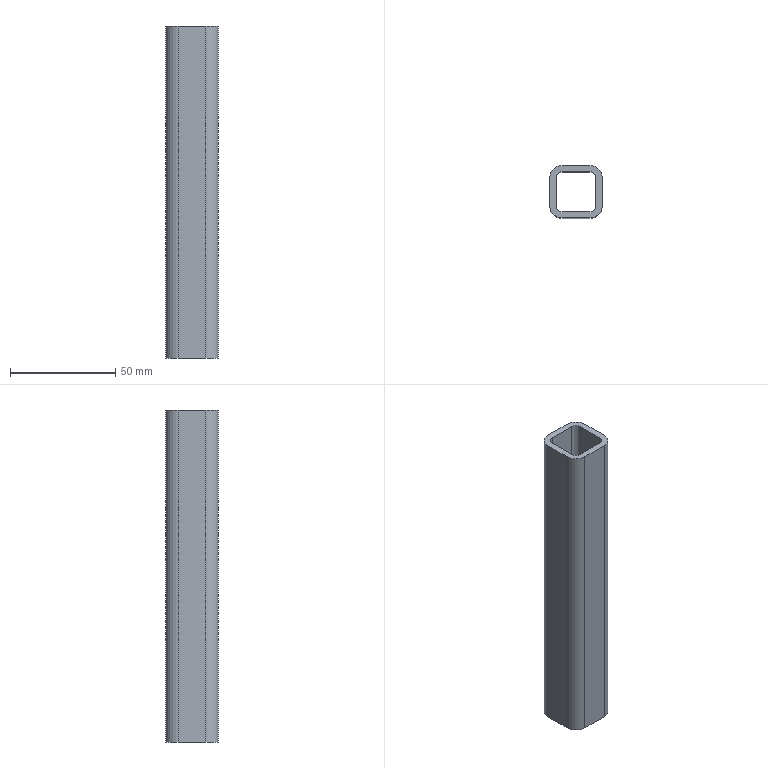Part | STEP file | ISO 10799-2 25x25x3 1784906820767 | 1 solid | 18 faces | box 25 x 25 x 158 mm | volume 38050 mm3 | plane 10 | cylinder 8 | commonest cylinder face diameters 6 x4 12 x4
STEP:
#1=CARTESIAN_POINT('',(-6.5,-9.5,183.));
#2=VERTEX_POINT('',#1);
#3=CARTESIAN_POINT('',(6.5,-9.5,183.));
#4=VERTEX_POINT('',#3);
#5=CARTESIAN_POINT('',(3.25,-9.5,183.));
#6=DIRECTION('',(1.,0.,0.));
#7=VECTOR('',#6,10.);
#8=LINE('',#5,#7);
#9=EDGE_CURVE('',#2,#4,#8,.T.);
#10=ORIENTED_EDGE('',*,*,#9,.T.);
#11=CARTESIAN_POINT('',(6.5,-9.5,25.));
#12=VERTEX_POINT('',#11);
#13=CARTESIAN_POINT('',(6.5,-9.5,0.));
#14=DIRECTION('',(0.,0.,1.));
#15=VECTOR('',#14,10.);
#16=LINE('',#13,#15);
#17=EDGE_CURVE('',#12,#4,#16,.T.);
#18=ORIENTED_EDGE('',*,*,#17,.F.);
#19=CARTESIAN_POINT('',(-6.5,-9.5,25.));
#20=VERTEX_POINT('',#19);
#21=CARTESIAN_POINT('',(3.25,-9.5,25.));
#22=DIRECTION('',(1.,0.,0.));
#23=VECTOR('',#22,10.);
#24=LINE('',#21,#23);
#25=EDGE_CURVE('',#20,#12,#24,.T.);
#26=ORIENTED_EDGE('',*,*,#25,.F.);
#27=CARTESIAN_POINT('',(-6.5,-9.5,0.));
#28=DIRECTION('',(0.,0.,1.));
#29=VECTOR('',#28,10.);
#30=LINE('',#27,#29);
#31=EDGE_CURVE('',#20,#2,#30,.T.);
#32=ORIENTED_EDGE('',*,*,#31,.T.);
#33=EDGE_LOOP('',(#10,#18,#26,#32));
#34=FACE_OUTER_BOUND('',#33,.T.);
#35=CARTESIAN_POINT('',(6.5,-9.5,0.));
#36=DIRECTION('',(0.,-1.,0.));
#37=DIRECTION('',(0.,0.,-1.));
#38=AXIS2_PLACEMENT_3D('',#35,#36,#37);
#39=PLANE('',#38);
#40=ADVANCED_FACE('',(#34),#39,.F.);
#41=CARTESIAN_POINT('',(9.5,-6.5,183.));
#42=VERTEX_POINT('',#41);
#43=CARTESIAN_POINT('',(6.5,-6.5,183.));
#44=DIRECTION('',(0.,0.,1.));
#45=DIRECTION('',(0.,1.,0.));
#46=AXIS2_PLACEMENT_3D('',#43,#44,#45);
#47=CIRCLE('',#46,3.);
#48=EDGE_CURVE('',#4,#42,#47,.T.);
#49=ORIENTED_EDGE('',*,*,#48,.T.);
#50=CARTESIAN_POINT('',(9.5,-6.5,25.));
#51=VERTEX_POINT('',#50);
#52=CARTESIAN_POINT('',(9.5,-6.5,0.));
#53=DIRECTION('',(0.,0.,1.));
#54=VECTOR('',#53,10.);
#55=LINE('',#52,#54);
#56=EDGE_CURVE('',#51,#42,#55,.T.);
#57=ORIENTED_EDGE('',*,*,#56,.F.);
#58=CARTESIAN_POINT('',(6.5,-6.5,25.));
#59=DIRECTION('',(0.,0.,1.));
#60=DIRECTION('',(0.,1.,0.));
#61=AXIS2_PLACEMENT_3D('',#58,#59,#60);
#62=CIRCLE('',#61,3.);
#63=EDGE_CURVE('',#12,#51,#62,.T.);
#64=ORIENTED_EDGE('',*,*,#63,.F.);
#65=ORIENTED_EDGE('',*,*,#17,.T.);
#66=EDGE_LOOP('',(#49,#57,#64,#65));
#67=FACE_OUTER_BOUND('',#66,.T.);
#68=CARTESIAN_POINT('',(6.5,-6.5,0.));
#69=DIRECTION('',(0.,0.,1.));
#70=DIRECTION('',(0.,1.,0.));
#71=AXIS2_PLACEMENT_3D('',#68,#69,#70);
#72=CYLINDRICAL_SURFACE('',#71,3.);
#73=ADVANCED_FACE('',(#67),#72,.F.);
#74=CARTESIAN_POINT('',(9.5,6.5,183.));
#75=VERTEX_POINT('',#74);
#76=CARTESIAN_POINT('',(9.5,3.25,183.));
#77=DIRECTION('',(0.,1.,0.));
#78=VECTOR('',#77,10.);
#79=LINE('',#76,#78);
#80=EDGE_CURVE('',#42,#75,#79,.T.);
#81=ORIENTED_EDGE('',*,*,#80,.T.);
#82=CARTESIAN_POINT('',(9.5,6.5,25.));
#83=VERTEX_POINT('',#82);
#84=CARTESIAN_POINT('',(9.5,6.5,0.));
#85=DIRECTION('',(0.,0.,1.));
#86=VECTOR('',#85,10.);
#87=LINE('',#84,#86);
#88=EDGE_CURVE('',#83,#75,#87,.T.);
#89=ORIENTED_EDGE('',*,*,#88,.F.);
#90=CARTESIAN_POINT('',(9.5,3.25,25.));
#91=DIRECTION('',(0.,1.,0.));
#92=VECTOR('',#91,10.);
#93=LINE('',#90,#92);
#94=EDGE_CURVE('',#51,#83,#93,.T.);
#95=ORIENTED_EDGE('',*,*,#94,.F.);
#96=ORIENTED_EDGE('',*,*,#56,.T.);
#97=EDGE_LOOP('',(#81,#89,#95,#96));
#98=FACE_OUTER_BOUND('',#97,.T.);
#99=CARTESIAN_POINT('',(9.5,6.5,0.));
#100=DIRECTION('',(1.,0.,0.));
#101=DIRECTION('',(0.,0.,-1.));
#102=AXIS2_PLACEMENT_3D('',#99,#100,#101);
#103=PLANE('',#102);
#104=ADVANCED_FACE('',(#98),#103,.F.);
#105=CARTESIAN_POINT('',(6.5,9.5,183.));
#106=VERTEX_POINT('',#105);
#107=CARTESIAN_POINT('',(6.5,6.5,183.));
#108=DIRECTION('',(0.,0.,1.));
#109=DIRECTION('',(-1.,0.,0.));
#110=AXIS2_PLACEMENT_3D('',#107,#108,#109);
#111=CIRCLE('',#110,3.);
#112=EDGE_CURVE('',#75,#106,#111,.T.);
#113=ORIENTED_EDGE('',*,*,#112,.T.);
#114=CARTESIAN_POINT('',(6.5,9.5,25.));
#115=VERTEX_POINT('',#114);
#116=CARTESIAN_POINT('',(6.5,9.5,0.));
#117=DIRECTION('',(0.,0.,1.));
#118=VECTOR('',#117,10.);
#119=LINE('',#116,#118);
#120=EDGE_CURVE('',#115,#106,#119,.T.);
#121=ORIENTED_EDGE('',*,*,#120,.F.);
#122=CARTESIAN_POINT('',(6.5,6.5,25.));
#123=DIRECTION('',(0.,0.,1.));
#124=DIRECTION('',(-1.,0.,0.));
#125=AXIS2_PLACEMENT_3D('',#122,#123,#124);
#126=CIRCLE('',#125,3.);
#127=EDGE_CURVE('',#83,#115,#126,.T.);
#128=ORIENTED_EDGE('',*,*,#127,.F.);
#129=ORIENTED_EDGE('',*,*,#88,.T.);
#130=EDGE_LOOP('',(#113,#121,#128,#129));
#131=FACE_OUTER_BOUND('',#130,.T.);
#132=CARTESIAN_POINT('',(6.5,6.5,0.));
#133=DIRECTION('',(0.,0.,1.));
#134=DIRECTION('',(-1.,0.,0.));
#135=AXIS2_PLACEMENT_3D('',#132,#133,#134);
#136=CYLINDRICAL_SURFACE('',#135,3.);
#137=ADVANCED_FACE('',(#131),#136,.F.);
#138=CARTESIAN_POINT('',(12.5,6.5,183.));
#139=VERTEX_POINT('',#138);
#140=CARTESIAN_POINT('',(12.5,-6.5,183.));
#141=VERTEX_POINT('',#140);
#142=CARTESIAN_POINT('',(12.5,3.25,183.));
#143=DIRECTION('',(0.,-1.,0.));
#144=VECTOR('',#143,10.);
#145=LINE('',#142,#144);
#146=EDGE_CURVE('',#139,#141,#145,.T.);
#147=ORIENTED_EDGE('',*,*,#146,.T.);
#148=CARTESIAN_POINT('',(12.5,-6.5,25.));
#149=VERTEX_POINT('',#148);
#150=CARTESIAN_POINT('',(12.5,-6.5,0.));
#151=DIRECTION('',(0.,0.,1.));
#152=VECTOR('',#151,10.);
#153=LINE('',#150,#152);
#154=EDGE_CURVE('',#149,#141,#153,.T.);
#155=ORIENTED_EDGE('',*,*,#154,.F.);
#156=CARTESIAN_POINT('',(12.5,6.5,25.));
#157=VERTEX_POINT('',#156);
#158=CARTESIAN_POINT('',(12.5,3.25,25.));
#159=DIRECTION('',(0.,-1.,0.));
#160=VECTOR('',#159,10.);
#161=LINE('',#158,#160);
#162=EDGE_CURVE('',#157,#149,#161,.T.);
#163=ORIENTED_EDGE('',*,*,#162,.F.);
#164=CARTESIAN_POINT('',(12.5,6.5,0.));
#165=DIRECTION('',(0.,0.,1.));
#166=VECTOR('',#165,10.);
#167=LINE('',#164,#166);
#168=EDGE_CURVE('',#157,#139,#167,.T.);
#169=ORIENTED_EDGE('',*,*,#168,.T.);
#170=EDGE_LOOP('',(#147,#155,#163,#169));
#171=FACE_OUTER_BOUND('',#170,.T.);
#172=CARTESIAN_POINT('',(12.5,6.5,0.));
#173=DIRECTION('',(1.,0.,0.));
#174=DIRECTION('',(0.,0.,-1.));
#175=AXIS2_PLACEMENT_3D('',#172,#173,#174);
#176=PLANE('',#175);
#177=ADVANCED_FACE('',(#171),#176,.T.);
#178=CARTESIAN_POINT('',(6.5,-12.5,183.));
#179=VERTEX_POINT('',#178);
#180=CARTESIAN_POINT('',(6.5,-6.5,183.));
#181=DIRECTION('',(0.,0.,-1.));
#182=DIRECTION('',(0.,1.,0.));
#183=AXIS2_PLACEMENT_3D('',#180,#181,#182);
#184=CIRCLE('',#183,6.);
#185=EDGE_CURVE('',#141,#179,#184,.T.);
#186=ORIENTED_EDGE('',*,*,#185,.T.);
#187=CARTESIAN_POINT('',(6.5,-12.5,25.));
#188=VERTEX_POINT('',#187);
#189=CARTESIAN_POINT('',(6.5,-12.5,0.));
#190=DIRECTION('',(0.,0.,1.));
#191=VECTOR('',#190,10.);
#192=LINE('',#189,#191);
#193=EDGE_CURVE('',#188,#179,#192,.T.);
#194=ORIENTED_EDGE('',*,*,#193,.F.);
#195=CARTESIAN_POINT('',(6.5,-6.5,25.));
#196=DIRECTION('',(0.,0.,-1.));
#197=DIRECTION('',(0.,1.,0.));
#198=AXIS2_PLACEMENT_3D('',#195,#196,#197);
#199=CIRCLE('',#198,6.);
#200=EDGE_CURVE('',#149,#188,#199,.T.);
#201=ORIENTED_EDGE('',*,*,#200,.F.);
#202=ORIENTED_EDGE('',*,*,#154,.T.);
#203=EDGE_LOOP('',(#186,#194,#201,#202));
#204=FACE_OUTER_BOUND('',#203,.T.);
#205=CARTESIAN_POINT('',(6.5,-6.5,0.));
#206=DIRECTION('',(0.,0.,1.));
#207=DIRECTION('',(0.,1.,0.));
#208=AXIS2_PLACEMENT_3D('',#205,#206,#207);
#209=CYLINDRICAL_SURFACE('',#208,6.);
#210=ADVANCED_FACE('',(#204),#209,.T.);
#211=CARTESIAN_POINT('',(-6.5,-12.5,183.));
#212=VERTEX_POINT('',#211);
#213=CARTESIAN_POINT('',(3.25,-12.5,183.));
#214=DIRECTION('',(-1.,0.,0.));
#215=VECTOR('',#214,10.);
#216=LINE('',#213,#215);
#217=EDGE_CURVE('',#179,#212,#216,.T.);
#218=ORIENTED_EDGE('',*,*,#217,.T.);
#219=CARTESIAN_POINT('',(-6.5,-12.5,25.));
#220=VERTEX_POINT('',#219);
#221=CARTESIAN_POINT('',(-6.5,-12.5,0.));
#222=DIRECTION('',(0.,0.,1.));
#223=VECTOR('',#222,10.);
#224=LINE('',#221,#223);
#225=EDGE_CURVE('',#220,#212,#224,.T.);
#226=ORIENTED_EDGE('',*,*,#225,.F.);
#227=CARTESIAN_POINT('',(3.25,-12.5,25.));
#228=DIRECTION('',(-1.,0.,0.));
#229=VECTOR('',#228,10.);
#230=LINE('',#227,#229);
#231=EDGE_CURVE('',#188,#220,#230,.T.);
#232=ORIENTED_EDGE('',*,*,#231,.F.);
#233=ORIENTED_EDGE('',*,*,#193,.T.);
#234=EDGE_LOOP('',(#218,#226,#232,#233));
#235=FACE_OUTER_BOUND('',#234,.T.);
#236=CARTESIAN_POINT('',(6.5,-12.5,0.));
#237=DIRECTION('',(0.,-1.,0.));
#238=DIRECTION('',(0.,0.,-1.));
#239=AXIS2_PLACEMENT_3D('',#236,#237,#238);
#240=PLANE('',#239);
#241=ADVANCED_FACE('',(#235),#240,.T.);
#242=CARTESIAN_POINT('',(-12.5,-6.5,183.));
#243=VERTEX_POINT('',#242);
#244=CARTESIAN_POINT('',(-6.5,-6.5,183.));
#245=DIRECTION('',(0.,0.,-1.));
#246=DIRECTION('',(1.,0.,0.));
#247=AXIS2_PLACEMENT_3D('',#244,#245,#246);
#248=CIRCLE('',#247,6.);
#249=EDGE_CURVE('',#212,#243,#248,.T.);
#250=ORIENTED_EDGE('',*,*,#249,.T.);
#251=CARTESIAN_POINT('',(-12.5,-6.5,25.));
#252=VERTEX_POINT('',#251);
#253=CARTESIAN_POINT('',(-12.5,-6.5,0.));
#254=DIRECTION('',(0.,0.,1.));
#255=VECTOR('',#254,10.);
#256=LINE('',#253,#255);
#257=EDGE_CURVE('',#252,#243,#256,.T.);
#258=ORIENTED_EDGE('',*,*,#257,.F.);
#259=CARTESIAN_POINT('',(-6.5,-6.5,25.));
#260=DIRECTION('',(0.,0.,-1.));
#261=DIRECTION('',(1.,0.,0.));
#262=AXIS2_PLACEMENT_3D('',#259,#260,#261);
#263=CIRCLE('',#262,6.);
#264=EDGE_CURVE('',#220,#252,#263,.T.);
#265=ORIENTED_EDGE('',*,*,#264,.F.);
#266=ORIENTED_EDGE('',*,*,#225,.T.);
#267=EDGE_LOOP('',(#250,#258,#265,#266));
#268=FACE_OUTER_BOUND('',#267,.T.);
#269=CARTESIAN_POINT('',(-6.5,-6.5,0.));
#270=DIRECTION('',(0.,0.,1.));
#271=DIRECTION('',(1.,0.,0.));
#272=AXIS2_PLACEMENT_3D('',#269,#270,#271);
#273=CYLINDRICAL_SURFACE('',#272,6.);
#274=ADVANCED_FACE('',(#268),#273,.T.);
#275=CARTESIAN_POINT('',(-6.5,9.5,183.));
#276=VERTEX_POINT('',#275);
#277=CARTESIAN_POINT('',(-3.25,9.5,183.));
#278=DIRECTION('',(-1.,0.,0.));
#279=VECTOR('',#278,10.);
#280=LINE('',#277,#279);
#281=EDGE_CURVE('',#106,#276,#280,.T.);
#282=ORIENTED_EDGE('',*,*,#281,.T.);
#283=CARTESIAN_POINT('',(-6.5,9.5,25.));
#284=VERTEX_POINT('',#283);
#285=CARTESIAN_POINT('',(-6.5,9.5,0.));
#286=DIRECTION('',(0.,0.,1.));
#287=VECTOR('',#286,10.);
#288=LINE('',#285,#287);
#289=EDGE_CURVE('',#284,#276,#288,.T.);
#290=ORIENTED_EDGE('',*,*,#289,.F.);
#291=CARTESIAN_POINT('',(-3.25,9.5,25.));
#292=DIRECTION('',(-1.,0.,0.));
#293=VECTOR('',#292,10.);
#294=LINE('',#291,#293);
#295=EDGE_CURVE('',#115,#284,#294,.T.);
#296=ORIENTED_EDGE('',*,*,#295,.F.);
#297=ORIENTED_EDGE('',*,*,#120,.T.);
#298=EDGE_LOOP('',(#282,#290,#296,#297));
#299=FACE_OUTER_BOUND('',#298,.T.);
#300=CARTESIAN_POINT('',(-6.5,9.5,0.));
#301=DIRECTION('',(0.,1.,0.));
#302=DIRECTION('',(0.,0.,1.));
#303=AXIS2_PLACEMENT_3D('',#300,#301,#302);
#304=PLANE('',#303);
#305=ADVANCED_FACE('',(#299),#304,.F.);
#306=CARTESIAN_POINT('',(-9.5,-6.5,183.));
#307=VERTEX_POINT('',#306);
#308=CARTESIAN_POINT('',(-6.5,-6.5,183.));
#309=DIRECTION('',(0.,0.,1.));
#310=DIRECTION('',(1.,0.,0.));
#311=AXIS2_PLACEMENT_3D('',#308,#309,#310);
#312=CIRCLE('',#311,3.);
#313=EDGE_CURVE('',#307,#2,#312,.T.);
#314=ORIENTED_EDGE('',*,*,#313,.T.);
#315=ORIENTED_EDGE('',*,*,#31,.F.);
#316=CARTESIAN_POINT('',(-9.5,-6.5,25.));
#317=VERTEX_POINT('',#316);
#318=CARTESIAN_POINT('',(-6.5,-6.5,25.));
#319=DIRECTION('',(0.,0.,1.));
#320=DIRECTION('',(1.,0.,0.));
#321=AXIS2_PLACEMENT_3D('',#318,#319,#320);
#322=CIRCLE('',#321,3.);
#323=EDGE_CURVE('',#317,#20,#322,.T.);
#324=ORIENTED_EDGE('',*,*,#323,.F.);
#325=CARTESIAN_POINT('',(-9.5,-6.5,0.));
#326=DIRECTION('',(0.,0.,1.));
#327=VECTOR('',#326,10.);
#328=LINE('',#325,#327);
#329=EDGE_CURVE('',#317,#307,#328,.T.);
#330=ORIENTED_EDGE('',*,*,#329,.T.);
#331=EDGE_LOOP('',(#314,#315,#324,#330));
#332=FACE_OUTER_BOUND('',#331,.T.);
#333=CARTESIAN_POINT('',(-6.5,-6.5,0.));
#334=DIRECTION('',(0.,0.,1.));
#335=DIRECTION('',(1.,0.,0.));
#336=AXIS2_PLACEMENT_3D('',#333,#334,#335);
#337=CYLINDRICAL_SURFACE('',#336,3.);
#338=ADVANCED_FACE('',(#332),#337,.F.);
#339=CARTESIAN_POINT('',(-9.5,6.5,183.));
#340=VERTEX_POINT('',#339);
#341=CARTESIAN_POINT('',(-9.5,-3.25,183.));
#342=DIRECTION('',(0.,-1.,0.));
#343=VECTOR('',#342,10.);
#344=LINE('',#341,#343);
#345=EDGE_CURVE('',#340,#307,#344,.T.);
#346=ORIENTED_EDGE('',*,*,#345,.T.);
#347=ORIENTED_EDGE('',*,*,#329,.F.);
#348=CARTESIAN_POINT('',(-9.5,6.5,25.));
#349=VERTEX_POINT('',#348);
#350=CARTESIAN_POINT('',(-9.5,-3.25,25.));
#351=DIRECTION('',(0.,-1.,0.));
#352=VECTOR('',#351,10.);
#353=LINE('',#350,#352);
#354=EDGE_CURVE('',#349,#317,#353,.T.);
#355=ORIENTED_EDGE('',*,*,#354,.F.);
#356=CARTESIAN_POINT('',(-9.5,6.5,0.));
#357=DIRECTION('',(0.,0.,1.));
#358=VECTOR('',#357,10.);
#359=LINE('',#356,#358);
#360=EDGE_CURVE('',#349,#340,#359,.T.);
#361=ORIENTED_EDGE('',*,*,#360,.T.);
#362=EDGE_LOOP('',(#346,#347,#355,#361));
#363=FACE_OUTER_BOUND('',#362,.T.);
#364=CARTESIAN_POINT('',(-9.5,-6.5,0.));
#365=DIRECTION('',(-1.,0.,0.));
#366=DIRECTION('',(0.,0.,1.));
#367=AXIS2_PLACEMENT_3D('',#364,#365,#366);
#368=PLANE('',#367);
#369=ADVANCED_FACE('',(#363),#368,.F.);
#370=CARTESIAN_POINT('',(-6.5,6.5,183.));
#371=DIRECTION('',(0.,0.,1.));
#372=DIRECTION('',(0.,-1.,0.));
#373=AXIS2_PLACEMENT_3D('',#370,#371,#372);
#374=CIRCLE('',#373,3.);
#375=EDGE_CURVE('',#276,#340,#374,.T.);
#376=ORIENTED_EDGE('',*,*,#375,.T.);
#377=ORIENTED_EDGE('',*,*,#360,.F.);
#378=CARTESIAN_POINT('',(-6.5,6.5,25.));
#379=DIRECTION('',(0.,0.,1.));
#380=DIRECTION('',(0.,-1.,0.));
#381=AXIS2_PLACEMENT_3D('',#378,#379,#380);
#382=CIRCLE('',#381,3.);
#383=EDGE_CURVE('',#284,#349,#382,.T.);
#384=ORIENTED_EDGE('',*,*,#383,.F.);
#385=ORIENTED_EDGE('',*,*,#289,.T.);
#386=EDGE_LOOP('',(#376,#377,#384,#385));
#387=FACE_OUTER_BOUND('',#386,.T.);
#388=CARTESIAN_POINT('',(-6.5,6.5,0.));
#389=DIRECTION('',(0.,0.,1.));
#390=DIRECTION('',(0.,-1.,0.));
#391=AXIS2_PLACEMENT_3D('',#388,#389,#390);
#392=CYLINDRICAL_SURFACE('',#391,3.);
#393=ADVANCED_FACE('',(#387),#392,.F.);
#394=CARTESIAN_POINT('',(-12.5,6.5,183.));
#395=VERTEX_POINT('',#394);
#396=CARTESIAN_POINT('',(-12.5,-3.25,183.));
#397=DIRECTION('',(0.,1.,0.));
#398=VECTOR('',#397,10.);
#399=LINE('',#396,#398);
#400=EDGE_CURVE('',#243,#395,#399,.T.);
#401=ORIENTED_EDGE('',*,*,#400,.T.);
#402=CARTESIAN_POINT('',(-12.5,6.5,25.));
#403=VERTEX_POINT('',#402);
#404=CARTESIAN_POINT('',(-12.5,6.5,0.));
#405=DIRECTION('',(0.,0.,1.));
#406=VECTOR('',#405,10.);
#407=LINE('',#404,#406);
#408=EDGE_CURVE('',#403,#395,#407,.T.);
#409=ORIENTED_EDGE('',*,*,#408,.F.);
#410=CARTESIAN_POINT('',(-12.5,-3.25,25.));
#411=DIRECTION('',(0.,1.,0.));
#412=VECTOR('',#411,10.);
#413=LINE('',#410,#412);
#414=EDGE_CURVE('',#252,#403,#413,.T.);
#415=ORIENTED_EDGE('',*,*,#414,.F.);
#416=ORIENTED_EDGE('',*,*,#257,.T.);
#417=EDGE_LOOP('',(#401,#409,#415,#416));
#418=FACE_OUTER_BOUND('',#417,.T.);
#419=CARTESIAN_POINT('',(-12.5,-6.5,0.));
#420=DIRECTION('',(-1.,0.,0.));
#421=DIRECTION('',(0.,0.,1.));
#422=AXIS2_PLACEMENT_3D('',#419,#420,#421);
#423=PLANE('',#422);
#424=ADVANCED_FACE('',(#418),#423,.T.);
#425=CARTESIAN_POINT('',(-6.5,12.5,183.));
#426=VERTEX_POINT('',#425);
#427=CARTESIAN_POINT('',(-6.5,6.5,183.));
#428=DIRECTION('',(0.,0.,-1.));
#429=DIRECTION('',(0.,-1.,0.));
#430=AXIS2_PLACEMENT_3D('',#427,#428,#429);
#431=CIRCLE('',#430,6.);
#432=EDGE_CURVE('',#395,#426,#431,.T.);
#433=ORIENTED_EDGE('',*,*,#432,.T.);
#434=CARTESIAN_POINT('',(-6.5,12.5,25.));
#435=VERTEX_POINT('',#434);
#436=CARTESIAN_POINT('',(-6.5,12.5,0.));
#437=DIRECTION('',(0.,0.,1.));
#438=VECTOR('',#437,10.);
#439=LINE('',#436,#438);
#440=EDGE_CURVE('',#435,#426,#439,.T.);
#441=ORIENTED_EDGE('',*,*,#440,.F.);
#442=CARTESIAN_POINT('',(-6.5,6.5,25.));
#443=DIRECTION('',(0.,0.,-1.));
#444=DIRECTION('',(0.,-1.,0.));
#445=AXIS2_PLACEMENT_3D('',#442,#443,#444);
#446=CIRCLE('',#445,6.);
#447=EDGE_CURVE('',#403,#435,#446,.T.);
#448=ORIENTED_EDGE('',*,*,#447,.F.);
#449=ORIENTED_EDGE('',*,*,#408,.T.);
#450=EDGE_LOOP('',(#433,#441,#448,#449));
#451=FACE_OUTER_BOUND('',#450,.T.);
#452=CARTESIAN_POINT('',(-6.5,6.5,0.));
#453=DIRECTION('',(0.,0.,1.));
#454=DIRECTION('',(0.,-1.,0.));
#455=AXIS2_PLACEMENT_3D('',#452,#453,#454);
#456=CYLINDRICAL_SURFACE('',#455,6.);
#457=ADVANCED_FACE('',(#451),#456,.T.);
#458=CARTESIAN_POINT('',(6.5,12.5,183.));
#459=VERTEX_POINT('',#458);
#460=CARTESIAN_POINT('',(-3.25,12.5,183.));
#461=DIRECTION('',(1.,0.,0.));
#462=VECTOR('',#461,10.);
#463=LINE('',#460,#462);
#464=EDGE_CURVE('',#426,#459,#463,.T.);
#465=ORIENTED_EDGE('',*,*,#464,.T.);
#466=CARTESIAN_POINT('',(6.5,12.5,25.));
#467=VERTEX_POINT('',#466);
#468=CARTESIAN_POINT('',(6.5,12.5,0.));
#469=DIRECTION('',(0.,0.,1.));
#470=VECTOR('',#469,10.);
#471=LINE('',#468,#470);
#472=EDGE_CURVE('',#467,#459,#471,.T.);
#473=ORIENTED_EDGE('',*,*,#472,.F.);
#474=CARTESIAN_POINT('',(-3.25,12.5,25.));
#475=DIRECTION('',(1.,0.,0.));
#476=VECTOR('',#475,10.);
#477=LINE('',#474,#476);
#478=EDGE_CURVE('',#435,#467,#477,.T.);
#479=ORIENTED_EDGE('',*,*,#478,.F.);
#480=ORIENTED_EDGE('',*,*,#440,.T.);
#481=EDGE_LOOP('',(#465,#473,#479,#480));
#482=FACE_OUTER_BOUND('',#481,.T.);
#483=CARTESIAN_POINT('',(-6.5,12.5,0.));
#484=DIRECTION('',(0.,1.,0.));
#485=DIRECTION('',(0.,0.,1.));
#486=AXIS2_PLACEMENT_3D('',#483,#484,#485);
#487=PLANE('',#486);
#488=ADVANCED_FACE('',(#482),#487,.T.);
#489=CARTESIAN_POINT('',(6.5,6.5,183.));
#490=DIRECTION('',(0.,0.,-1.));
#491=DIRECTION('',(-1.,0.,0.));
#492=AXIS2_PLACEMENT_3D('',#489,#490,#491);
#493=CIRCLE('',#492,6.);
#494=EDGE_CURVE('',#459,#139,#493,.T.);
#495=ORIENTED_EDGE('',*,*,#494,.T.);
#496=ORIENTED_EDGE('',*,*,#168,.F.);
#497=CARTESIAN_POINT('',(6.5,6.5,25.));
#498=DIRECTION('',(0.,0.,-1.));
#499=DIRECTION('',(-1.,0.,0.));
#500=AXIS2_PLACEMENT_3D('',#497,#498,#499);
#501=CIRCLE('',#500,6.);
#502=EDGE_CURVE('',#467,#157,#501,.T.);
#503=ORIENTED_EDGE('',*,*,#502,.F.);
#504=ORIENTED_EDGE('',*,*,#472,.T.);
#505=EDGE_LOOP('',(#495,#496,#503,#504));
#506=FACE_OUTER_BOUND('',#505,.T.);
#507=CARTESIAN_POINT('',(6.5,6.5,0.));
#508=DIRECTION('',(0.,0.,1.));
#509=DIRECTION('',(-1.,0.,0.));
#510=AXIS2_PLACEMENT_3D('',#507,#508,#509);
#511=CYLINDRICAL_SURFACE('',#510,6.);
#512=ADVANCED_FACE('',(#506),#511,.T.);
#513=ORIENTED_EDGE('',*,*,#414,.T.);
#514=ORIENTED_EDGE('',*,*,#447,.T.);
#515=ORIENTED_EDGE('',*,*,#478,.T.);
#516=ORIENTED_EDGE('',*,*,#502,.T.);
#517=ORIENTED_EDGE('',*,*,#162,.T.);
#518=ORIENTED_EDGE('',*,*,#200,.T.);
#519=ORIENTED_EDGE('',*,*,#231,.T.);
#520=ORIENTED_EDGE('',*,*,#264,.T.);
#521=EDGE_LOOP('',(#513,#514,#515,#516,#517,#518,#519,#520));
#522=FACE_OUTER_BOUND('',#521,.T.);
#523=ORIENTED_EDGE('',*,*,#295,.T.);
#524=ORIENTED_EDGE('',*,*,#383,.T.);
#525=ORIENTED_EDGE('',*,*,#354,.T.);
#526=ORIENTED_EDGE('',*,*,#323,.T.);
#527=ORIENTED_EDGE('',*,*,#25,.T.);
#528=ORIENTED_EDGE('',*,*,#63,.T.);
#529=ORIENTED_EDGE('',*,*,#94,.T.);
#530=ORIENTED_EDGE('',*,*,#127,.T.);
#531=EDGE_LOOP('',(#523,#524,#525,#526,#527,#528,#529,#530));
#532=FACE_BOUND('',#531,.T.);
#533=CARTESIAN_POINT('',(0.,0.,25.));
#534=DIRECTION('',(0.,0.,1.));
#535=DIRECTION('',(1.,0.,0.));
#536=AXIS2_PLACEMENT_3D('',#533,#534,#535);
#537=PLANE('',#536);
#538=ADVANCED_FACE('',(#522,#532),#537,.F.);
#539=ORIENTED_EDGE('',*,*,#400,.F.);
#540=ORIENTED_EDGE('',*,*,#249,.F.);
#541=ORIENTED_EDGE('',*,*,#217,.F.);
#542=ORIENTED_EDGE('',*,*,#185,.F.);
#543=ORIENTED_EDGE('',*,*,#146,.F.);
#544=ORIENTED_EDGE('',*,*,#494,.F.);
#545=ORIENTED_EDGE('',*,*,#464,.F.);
#546=ORIENTED_EDGE('',*,*,#432,.F.);
#547=EDGE_LOOP('',(#539,#540,#541,#542,#543,#544,#545,#546));
#548=FACE_OUTER_BOUND('',#547,.T.);
#549=ORIENTED_EDGE('',*,*,#281,.F.);
#550=ORIENTED_EDGE('',*,*,#112,.F.);
#551=ORIENTED_EDGE('',*,*,#80,.F.);
#552=ORIENTED_EDGE('',*,*,#48,.F.);
#553=ORIENTED_EDGE('',*,*,#9,.F.);
#554=ORIENTED_EDGE('',*,*,#313,.F.);
#555=ORIENTED_EDGE('',*,*,#345,.F.);
#556=ORIENTED_EDGE('',*,*,#375,.F.);
#557=EDGE_LOOP('',(#549,#550,#551,#552,#553,#554,#555,#556));
#558=FACE_BOUND('',#557,.T.);
#559=CARTESIAN_POINT('',(0.,0.,183.));
#560=DIRECTION('',(0.,0.,1.));
#561=DIRECTION('',(1.,0.,0.));
#562=AXIS2_PLACEMENT_3D('',#559,#560,#561);
#563=PLANE('',#562);
#564=ADVANCED_FACE('',(#548,#558),#563,.T.);
#565=CLOSED_SHELL('',(#40,#73,#104,#137,#177,#210,#241,#274,#305,#338,#369,#393,#424,#457,#488,#512,#538,#564));
#566=MANIFOLD_SOLID_BREP('',#565);
#567=(LENGTH_UNIT()NAMED_UNIT(*)SI_UNIT(.MILLI.,.METRE.));
#568=UNCERTAINTY_MEASURE_WITH_UNIT(LENGTH_MEASURE(0.01),#567,'','');
#569=(NAMED_UNIT(*)PLANE_ANGLE_UNIT()SI_UNIT($,.RADIAN.));
#570=(NAMED_UNIT(*)SI_UNIT($,.STERADIAN.)SOLID_ANGLE_UNIT());
#571=(GEOMETRIC_REPRESENTATION_CONTEXT(3)GLOBAL_UNCERTAINTY_ASSIGNED_CONTEXT((#568))GLOBAL_UNIT_ASSIGNED_CONTEXT((#567,#569,#570))REPRESENTATION_CONTEXT('',''));
#572=ADVANCED_BREP_SHAPE_REPRESENTATION('',(#566),#571);